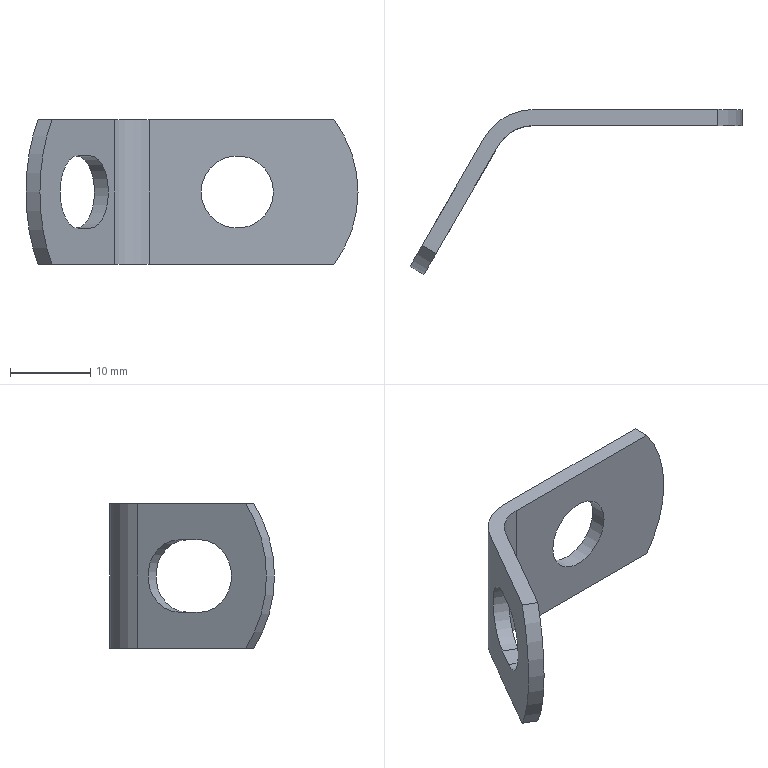Part | NX | features ACO1606-2-04 2 | 1 solid | 15 faces | box 41.25 x 20.486 x 18 mm | volume 1448 mm3 | plane 8 | cylinder 7 | commonest cylinder face diameters 9 x3 30 x2 10 x1 14 x1
STEP:
#1=CARTESIAN_POINT('',(-1007.011,-540.,-159.));
#2=VERTEX_POINT('',#1);
#3=CARTESIAN_POINT('',(-1007.011,-540.,-141.));
#4=VERTEX_POINT('',#3);
#5=CARTESIAN_POINT('',(-1007.011,-540.,-150.));
#6=DIRECTION('',(0.,0.,1.));
#7=VECTOR('',#6,1000.);
#8=LINE('',#5,#7);
#9=EDGE_CURVE('',#2,#4,#8,.T.);
#10=ORIENTED_EDGE('',*,*,#9,.T.);
#11=CARTESIAN_POINT('',(-1000.949,-536.5,-141.));
#12=VERTEX_POINT('',#11);
#13=CARTESIAN_POINT('',(-1000.949,-543.5,-141.));
#14=DIRECTION('',(0.,0.,-1.));
#15=DIRECTION('',(1.,0.,0.));
#16=AXIS2_PLACEMENT_3D('',#13,#14,#15);
#17=CIRCLE('',#16,7.);
#18=EDGE_CURVE('',#4,#12,#17,.T.);
#19=ORIENTED_EDGE('',*,*,#18,.T.);
#20=CARTESIAN_POINT('',(-1000.949,-536.5,-159.));
#21=VERTEX_POINT('',#20);
#22=CARTESIAN_POINT('',(-1000.949,-536.5,-150.));
#23=DIRECTION('',(0.,0.,1.));
#24=VECTOR('',#23,1000.);
#25=LINE('',#22,#24);
#26=EDGE_CURVE('',#21,#12,#25,.T.);
#27=ORIENTED_EDGE('',*,*,#26,.F.);
#28=CARTESIAN_POINT('',(-1000.949,-543.5,-159.));
#29=DIRECTION('',(0.,0.,-1.));
#30=DIRECTION('',(1.,0.,0.));
#31=AXIS2_PLACEMENT_3D('',#28,#29,#30);
#32=CIRCLE('',#31,7.);
#33=EDGE_CURVE('',#2,#21,#32,.T.);
#34=ORIENTED_EDGE('',*,*,#33,.F.);
#35=EDGE_LOOP('',(#10,#19,#27,#34));
#36=FACE_BOUND('',#35,.T.);
#37=CARTESIAN_POINT('',(-1000.949,-543.5,-150.));
#38=DIRECTION('',(0.,0.,1.));
#39=DIRECTION('',(1.,0.,0.));
#40=AXIS2_PLACEMENT_3D('',#37,#38,#39);
#41=CYLINDRICAL_SURFACE('',#40,7.);
#42=ADVANCED_FACE('',(#36),#41,.T.);
#43=CARTESIAN_POINT('',(-1014.74,-553.387,-159.));
#44=VERTEX_POINT('',#43);
#45=CARTESIAN_POINT('',(-1010.876,-546.694,-159.));
#46=DIRECTION('',(0.5,0.866,0.));
#47=VECTOR('',#46,1000.);
#48=LINE('',#45,#47);
#49=EDGE_CURVE('',#44,#2,#48,.T.);
#50=ORIENTED_EDGE('',*,*,#49,.F.);
#51=CARTESIAN_POINT('',(-1014.74,-553.387,-141.));
#52=VERTEX_POINT('',#51);
#53=CARTESIAN_POINT('',(-1008.74,-542.995,-150.));
#54=DIRECTION('',(0.866,-0.5,0.));
#55=DIRECTION('',(0.5,0.866,0.));
#56=AXIS2_PLACEMENT_3D('',#53,#54,#55);
#57=CIRCLE('',#56,15.);
#58=EDGE_CURVE('',#52,#44,#57,.T.);
#59=ORIENTED_EDGE('',*,*,#58,.F.);
#60=CARTESIAN_POINT('',(-1010.876,-546.694,-141.));
#61=DIRECTION('',(0.5,0.866,0.));
#62=VECTOR('',#61,1000.);
#63=LINE('',#60,#62);
#64=EDGE_CURVE('',#52,#4,#63,.T.);
#65=ORIENTED_EDGE('',*,*,#64,.T.);
#66=ORIENTED_EDGE('',*,*,#9,.F.);
#67=EDGE_LOOP('',(#50,#59,#65,#66));
#68=FACE_BOUND('',#67,.T.);
#69=CARTESIAN_POINT('',(-1011.49,-547.758,-145.5));
#70=VERTEX_POINT('',#69);
#71=CARTESIAN_POINT('',(-1009.99,-545.16,-145.5));
#72=VERTEX_POINT('',#71);
#73=CARTESIAN_POINT('',(-1010.74,-546.459,-145.5));
#74=DIRECTION('',(0.5,0.866,0.));
#75=VECTOR('',#74,1000.);
#76=LINE('',#73,#75);
#77=EDGE_CURVE('',#70,#72,#76,.T.);
#78=ORIENTED_EDGE('',*,*,#77,.F.);
#79=CARTESIAN_POINT('',(-1011.49,-547.758,-154.5));
#80=VERTEX_POINT('',#79);
#81=CARTESIAN_POINT('',(-1011.49,-547.758,-150.));
#82=DIRECTION('',(-0.866,0.5,0.));
#83=DIRECTION('',(0.5,0.866,0.));
#84=AXIS2_PLACEMENT_3D('',#81,#82,#83);
#85=CIRCLE('',#84,4.5);
#86=EDGE_CURVE('',#80,#70,#85,.T.);
#87=ORIENTED_EDGE('',*,*,#86,.F.);
#88=CARTESIAN_POINT('',(-1009.99,-545.16,-154.5));
#89=VERTEX_POINT('',#88);
#90=CARTESIAN_POINT('',(-1010.74,-546.459,-154.5));
#91=DIRECTION('',(-0.5,-0.866,0.));
#92=VECTOR('',#91,1000.);
#93=LINE('',#90,#92);
#94=EDGE_CURVE('',#89,#80,#93,.T.);
#95=ORIENTED_EDGE('',*,*,#94,.F.);
#96=CARTESIAN_POINT('',(-1009.99,-545.16,-150.));
#97=DIRECTION('',(-0.866,0.5,0.));
#98=DIRECTION('',(0.5,0.866,0.));
#99=AXIS2_PLACEMENT_3D('',#96,#97,#98);
#100=CIRCLE('',#99,4.5);
#101=EDGE_CURVE('',#72,#89,#100,.T.);
#102=ORIENTED_EDGE('',*,*,#101,.F.);
#103=EDGE_LOOP('',(#78,#87,#95,#102));
#104=FACE_BOUND('',#103,.T.);
#105=CARTESIAN_POINT('',(-1016.49,-556.419,-150.));
#106=DIRECTION('',(-0.866,0.5,0.));
#107=DIRECTION('',(0.5,0.866,0.));
#108=AXIS2_PLACEMENT_3D('',#105,#106,#107);
#109=PLANE('',#108);
#110=ADVANCED_FACE('',(#68,#104),#109,.T.);
#111=CARTESIAN_POINT('',(-977.99,-538.5,-159.));
#112=VERTEX_POINT('',#111);
#113=CARTESIAN_POINT('',(-977.99,-536.5,-159.));
#114=VERTEX_POINT('',#113);
#115=CARTESIAN_POINT('',(-977.99,-537.5,-159.));
#116=DIRECTION('',(0.,1.,0.));
#117=VECTOR('',#116,1000.);
#118=LINE('',#115,#117);
#119=EDGE_CURVE('',#112,#114,#118,.T.);
#120=ORIENTED_EDGE('',*,*,#119,.F.);
#121=CARTESIAN_POINT('',(-1000.949,-538.5,-159.));
#122=VERTEX_POINT('',#121);
#123=CARTESIAN_POINT('',(-989.47,-538.5,-159.));
#124=DIRECTION('',(-1.,0.,0.));
#125=VECTOR('',#124,1000.);
#126=LINE('',#123,#125);
#127=EDGE_CURVE('',#112,#122,#126,.T.);
#128=ORIENTED_EDGE('',*,*,#127,.T.);
#129=CARTESIAN_POINT('',(-1005.279,-541.,-159.));
#130=VERTEX_POINT('',#129);
#131=CARTESIAN_POINT('',(-1000.949,-543.5,-159.));
#132=DIRECTION('',(0.,0.,1.));
#133=DIRECTION('',(1.,0.,0.));
#134=AXIS2_PLACEMENT_3D('',#131,#132,#133);
#135=CIRCLE('',#134,5.);
#136=EDGE_CURVE('',#122,#130,#135,.T.);
#137=ORIENTED_EDGE('',*,*,#136,.T.);
#138=CARTESIAN_POINT('',(-1013.008,-554.387,-159.));
#139=VERTEX_POINT('',#138);
#140=CARTESIAN_POINT('',(-1009.144,-547.694,-159.));
#141=DIRECTION('',(-0.5,-0.866,0.));
#142=VECTOR('',#141,1000.);
#143=LINE('',#140,#142);
#144=EDGE_CURVE('',#130,#139,#143,.T.);
#145=ORIENTED_EDGE('',*,*,#144,.T.);
#146=CARTESIAN_POINT('',(-1013.874,-553.887,-159.));
#147=DIRECTION('',(-0.866,0.5,0.));
#148=VECTOR('',#147,1000.);
#149=LINE('',#146,#148);
#150=EDGE_CURVE('',#139,#44,#149,.T.);
#151=ORIENTED_EDGE('',*,*,#150,.T.);
#152=ORIENTED_EDGE('',*,*,#49,.T.);
#153=ORIENTED_EDGE('',*,*,#33,.T.);
#154=CARTESIAN_POINT('',(-989.47,-536.5,-159.));
#155=DIRECTION('',(1.,0.,0.));
#156=VECTOR('',#155,1000.);
#157=LINE('',#154,#156);
#158=EDGE_CURVE('',#21,#114,#157,.T.);
#159=ORIENTED_EDGE('',*,*,#158,.T.);
#160=EDGE_LOOP('',(#120,#128,#137,#145,#151,#152,#153,#159));
#161=FACE_BOUND('',#160,.T.);
#162=CARTESIAN_POINT('',(-1014.667,-527.579,-159.));
#163=DIRECTION('',(0.,0.,1.));
#164=DIRECTION('',(1.,0.,0.));
#165=AXIS2_PLACEMENT_3D('',#162,#163,#164);
#166=PLANE('',#165);
#167=ADVANCED_FACE('',(#161),#166,.F.);
#168=CARTESIAN_POINT('',(-977.99,-536.5,-141.));
#169=VERTEX_POINT('',#168);
#170=CARTESIAN_POINT('',(-989.99,-536.5,-150.));
#171=DIRECTION('',(0.,-1.,0.));
#172=DIRECTION('',(1.,0.,0.));
#173=AXIS2_PLACEMENT_3D('',#170,#171,#172);
#174=CIRCLE('',#173,15.);
#175=EDGE_CURVE('',#114,#169,#174,.T.);
#176=ORIENTED_EDGE('',*,*,#175,.F.);
#177=ORIENTED_EDGE('',*,*,#158,.F.);
#178=ORIENTED_EDGE('',*,*,#26,.T.);
#179=CARTESIAN_POINT('',(-989.47,-536.5,-141.));
#180=DIRECTION('',(1.,0.,0.));
#181=VECTOR('',#180,1000.);
#182=LINE('',#179,#181);
#183=EDGE_CURVE('',#12,#169,#182,.T.);
#184=ORIENTED_EDGE('',*,*,#183,.T.);
#185=EDGE_LOOP('',(#176,#177,#178,#184));
#186=FACE_BOUND('',#185,.T.);
#187=CARTESIAN_POINT('',(-985.49,-536.5,-150.));
#188=VERTEX_POINT('',#187);
#189=CARTESIAN_POINT('',(-989.99,-536.5,-150.));
#190=DIRECTION('',(0.,1.,0.));
#191=DIRECTION('',(1.,0.,0.));
#192=AXIS2_PLACEMENT_3D('',#189,#190,#191);
#193=CIRCLE('',#192,4.5);
#194=EDGE_CURVE('',#188,#188,#193,.T.);
#195=ORIENTED_EDGE('',*,*,#194,.F.);
#196=EDGE_LOOP('',(#195));
#197=FACE_BOUND('',#196,.T.);
#198=CARTESIAN_POINT('',(-1000.949,-536.5,-150.));
#199=DIRECTION('',(0.,1.,0.));
#200=DIRECTION('',(0.,0.,-1.));
#201=AXIS2_PLACEMENT_3D('',#198,#199,#200);
#202=PLANE('',#201);
#203=ADVANCED_FACE('',(#186,#197),#202,.T.);
#204=CARTESIAN_POINT('',(-977.99,-538.5,-141.));
#205=VERTEX_POINT('',#204);
#206=CARTESIAN_POINT('',(-1000.949,-538.5,-141.));
#207=VERTEX_POINT('',#206);
#208=CARTESIAN_POINT('',(-989.47,-538.5,-141.));
#209=DIRECTION('',(-1.,0.,0.));
#210=VECTOR('',#209,1000.);
#211=LINE('',#208,#210);
#212=EDGE_CURVE('',#205,#207,#211,.T.);
#213=ORIENTED_EDGE('',*,*,#212,.F.);
#214=CARTESIAN_POINT('',(-977.99,-537.5,-141.));
#215=DIRECTION('',(0.,1.,0.));
#216=VECTOR('',#215,1000.);
#217=LINE('',#214,#216);
#218=EDGE_CURVE('',#205,#169,#217,.T.);
#219=ORIENTED_EDGE('',*,*,#218,.T.);
#220=ORIENTED_EDGE('',*,*,#183,.F.);
#221=ORIENTED_EDGE('',*,*,#18,.F.);
#222=ORIENTED_EDGE('',*,*,#64,.F.);
#223=CARTESIAN_POINT('',(-1013.008,-554.387,-141.));
#224=VERTEX_POINT('',#223);
#225=CARTESIAN_POINT('',(-1013.874,-553.887,-141.));
#226=DIRECTION('',(-0.866,0.5,0.));
#227=VECTOR('',#226,1000.);
#228=LINE('',#225,#227);
#229=EDGE_CURVE('',#224,#52,#228,.T.);
#230=ORIENTED_EDGE('',*,*,#229,.F.);
#231=CARTESIAN_POINT('',(-1005.279,-541.,-141.));
#232=VERTEX_POINT('',#231);
#233=CARTESIAN_POINT('',(-1009.144,-547.694,-141.));
#234=DIRECTION('',(-0.5,-0.866,0.));
#235=VECTOR('',#234,1000.);
#236=LINE('',#233,#235);
#237=EDGE_CURVE('',#232,#224,#236,.T.);
#238=ORIENTED_EDGE('',*,*,#237,.F.);
#239=CARTESIAN_POINT('',(-1000.949,-543.5,-141.));
#240=DIRECTION('',(0.,0.,1.));
#241=DIRECTION('',(1.,0.,0.));
#242=AXIS2_PLACEMENT_3D('',#239,#240,#241);
#243=CIRCLE('',#242,5.);
#244=EDGE_CURVE('',#207,#232,#243,.T.);
#245=ORIENTED_EDGE('',*,*,#244,.F.);
#246=EDGE_LOOP('',(#213,#219,#220,#221,#222,#230,#238,#245));
#247=FACE_BOUND('',#246,.T.);
#248=CARTESIAN_POINT('',(-1014.667,-527.579,-141.));
#249=DIRECTION('',(0.,0.,1.));
#250=DIRECTION('',(1.,0.,0.));
#251=AXIS2_PLACEMENT_3D('',#248,#249,#250);
#252=PLANE('',#251);
#253=ADVANCED_FACE('',(#247),#252,.T.);
#254=ORIENTED_EDGE('',*,*,#229,.T.);
#255=ORIENTED_EDGE('',*,*,#58,.T.);
#256=ORIENTED_EDGE('',*,*,#150,.F.);
#257=CARTESIAN_POINT('',(-1007.008,-543.995,-150.));
#258=DIRECTION('',(0.866,-0.5,0.));
#259=DIRECTION('',(0.5,0.866,0.));
#260=AXIS2_PLACEMENT_3D('',#257,#258,#259);
#261=CIRCLE('',#260,15.);
#262=EDGE_CURVE('',#224,#139,#261,.T.);
#263=ORIENTED_EDGE('',*,*,#262,.F.);
#264=EDGE_LOOP('',(#254,#255,#256,#263));
#265=FACE_BOUND('',#264,.T.);
#266=CARTESIAN_POINT('',(-1007.874,-543.495,-150.));
#267=DIRECTION('',(0.866,-0.5,0.));
#268=DIRECTION('',(-0.5,-0.866,0.));
#269=AXIS2_PLACEMENT_3D('',#266,#267,#268);
#270=CYLINDRICAL_SURFACE('',#269,15.);
#271=ADVANCED_FACE('',(#265),#270,.T.);
#272=CARTESIAN_POINT('',(-1009.758,-548.758,-145.5));
#273=VERTEX_POINT('',#272);
#274=CARTESIAN_POINT('',(-1010.624,-548.258,-145.5));
#275=DIRECTION('',(-0.866,0.5,0.));
#276=VECTOR('',#275,1000.);
#277=LINE('',#274,#276);
#278=EDGE_CURVE('',#273,#70,#277,.T.);
#279=ORIENTED_EDGE('',*,*,#278,.T.);
#280=ORIENTED_EDGE('',*,*,#77,.T.);
#281=CARTESIAN_POINT('',(-1008.258,-546.16,-145.5));
#282=VERTEX_POINT('',#281);
#283=CARTESIAN_POINT('',(-1009.124,-545.66,-145.5));
#284=DIRECTION('',(-0.866,0.5,0.));
#285=VECTOR('',#284,1000.);
#286=LINE('',#283,#285);
#287=EDGE_CURVE('',#282,#72,#286,.T.);
#288=ORIENTED_EDGE('',*,*,#287,.F.);
#289=CARTESIAN_POINT('',(-1009.008,-547.459,-145.5));
#290=DIRECTION('',(0.5,0.866,0.));
#291=VECTOR('',#290,1000.);
#292=LINE('',#289,#291);
#293=EDGE_CURVE('',#273,#282,#292,.T.);
#294=ORIENTED_EDGE('',*,*,#293,.F.);
#295=EDGE_LOOP('',(#279,#280,#288,#294));
#296=FACE_BOUND('',#295,.T.);
#297=CARTESIAN_POINT('',(-1008.258,-546.16,-145.5));
#298=DIRECTION('',(0.,0.,1.));
#299=DIRECTION('',(1.,0.,0.));
#300=AXIS2_PLACEMENT_3D('',#297,#298,#299);
#301=PLANE('',#300);
#302=ADVANCED_FACE('',(#296),#301,.F.);
#303=ORIENTED_EDGE('',*,*,#287,.T.);
#304=ORIENTED_EDGE('',*,*,#101,.T.);
#305=CARTESIAN_POINT('',(-1008.258,-546.16,-154.5));
#306=VERTEX_POINT('',#305);
#307=CARTESIAN_POINT('',(-1009.124,-545.66,-154.5));
#308=DIRECTION('',(-0.866,0.5,0.));
#309=VECTOR('',#308,1000.);
#310=LINE('',#307,#309);
#311=EDGE_CURVE('',#306,#89,#310,.T.);
#312=ORIENTED_EDGE('',*,*,#311,.F.);
#313=CARTESIAN_POINT('',(-1008.258,-546.16,-150.));
#314=DIRECTION('',(-0.866,0.5,0.));
#315=DIRECTION('',(0.5,0.866,0.));
#316=AXIS2_PLACEMENT_3D('',#313,#314,#315);
#317=CIRCLE('',#316,4.5);
#318=EDGE_CURVE('',#282,#306,#317,.T.);
#319=ORIENTED_EDGE('',*,*,#318,.F.);
#320=EDGE_LOOP('',(#303,#304,#312,#319));
#321=FACE_BOUND('',#320,.T.);
#322=CARTESIAN_POINT('',(-1009.124,-545.66,-150.));
#323=DIRECTION('',(0.866,-0.5,0.));
#324=DIRECTION('',(-0.5,-0.866,0.));
#325=AXIS2_PLACEMENT_3D('',#322,#323,#324);
#326=CYLINDRICAL_SURFACE('',#325,4.5);
#327=ADVANCED_FACE('',(#321),#326,.F.);
#328=ORIENTED_EDGE('',*,*,#311,.T.);
#329=ORIENTED_EDGE('',*,*,#94,.T.);
#330=CARTESIAN_POINT('',(-1009.758,-548.758,-154.5));
#331=VERTEX_POINT('',#330);
#332=CARTESIAN_POINT('',(-1010.624,-548.258,-154.5));
#333=DIRECTION('',(-0.866,0.5,0.));
#334=VECTOR('',#333,1000.);
#335=LINE('',#332,#334);
#336=EDGE_CURVE('',#331,#80,#335,.T.);
#337=ORIENTED_EDGE('',*,*,#336,.F.);
#338=CARTESIAN_POINT('',(-1009.008,-547.459,-154.5));
#339=DIRECTION('',(-0.5,-0.866,0.));
#340=VECTOR('',#339,1000.);
#341=LINE('',#338,#340);
#342=EDGE_CURVE('',#306,#331,#341,.T.);
#343=ORIENTED_EDGE('',*,*,#342,.F.);
#344=EDGE_LOOP('',(#328,#329,#337,#343));
#345=FACE_BOUND('',#344,.T.);
#346=CARTESIAN_POINT('',(-1009.758,-548.758,-154.5));
#347=DIRECTION('',(0.,0.,-1.));
#348=DIRECTION('',(-1.,0.,0.));
#349=AXIS2_PLACEMENT_3D('',#346,#347,#348);
#350=PLANE('',#349);
#351=ADVANCED_FACE('',(#345),#350,.F.);
#352=ORIENTED_EDGE('',*,*,#336,.T.);
#353=ORIENTED_EDGE('',*,*,#86,.T.);
#354=ORIENTED_EDGE('',*,*,#278,.F.);
#355=CARTESIAN_POINT('',(-1009.758,-548.758,-150.));
#356=DIRECTION('',(-0.866,0.5,0.));
#357=DIRECTION('',(0.5,0.866,0.));
#358=AXIS2_PLACEMENT_3D('',#355,#356,#357);
#359=CIRCLE('',#358,4.5);
#360=EDGE_CURVE('',#331,#273,#359,.T.);
#361=ORIENTED_EDGE('',*,*,#360,.F.);
#362=EDGE_LOOP('',(#352,#353,#354,#361));
#363=FACE_BOUND('',#362,.T.);
#364=CARTESIAN_POINT('',(-1010.624,-548.258,-150.));
#365=DIRECTION('',(0.866,-0.5,0.));
#366=DIRECTION('',(-0.5,-0.866,0.));
#367=AXIS2_PLACEMENT_3D('',#364,#365,#366);
#368=CYLINDRICAL_SURFACE('',#367,4.5);
#369=ADVANCED_FACE('',(#363),#368,.F.);
#370=ORIENTED_EDGE('',*,*,#127,.F.);
#371=CARTESIAN_POINT('',(-989.99,-538.5,-150.));
#372=DIRECTION('',(0.,-1.,0.));
#373=DIRECTION('',(1.,0.,0.));
#374=AXIS2_PLACEMENT_3D('',#371,#372,#373);
#375=CIRCLE('',#374,15.);
#376=EDGE_CURVE('',#112,#205,#375,.T.);
#377=ORIENTED_EDGE('',*,*,#376,.T.);
#378=ORIENTED_EDGE('',*,*,#212,.T.);
#379=CARTESIAN_POINT('',(-1000.949,-538.5,-150.));
#380=DIRECTION('',(0.,0.,1.));
#381=VECTOR('',#380,1000.);
#382=LINE('',#379,#381);
#383=EDGE_CURVE('',#122,#207,#382,.T.);
#384=ORIENTED_EDGE('',*,*,#383,.F.);
#385=EDGE_LOOP('',(#370,#377,#378,#384));
#386=FACE_BOUND('',#385,.T.);
#387=CARTESIAN_POINT('',(-985.49,-538.5,-150.));
#388=VERTEX_POINT('',#387);
#389=CARTESIAN_POINT('',(-989.99,-538.5,-150.));
#390=DIRECTION('',(0.,1.,0.));
#391=DIRECTION('',(1.,0.,0.));
#392=AXIS2_PLACEMENT_3D('',#389,#390,#391);
#393=CIRCLE('',#392,4.5);
#394=EDGE_CURVE('',#388,#388,#393,.T.);
#395=ORIENTED_EDGE('',*,*,#394,.T.);
#396=EDGE_LOOP('',(#395));
#397=FACE_BOUND('',#396,.T.);
#398=CARTESIAN_POINT('',(-974.99,-538.5,-150.));
#399=DIRECTION('',(0.,-1.,0.));
#400=DIRECTION('',(0.,0.,1.));
#401=AXIS2_PLACEMENT_3D('',#398,#399,#400);
#402=PLANE('',#401);
#403=ADVANCED_FACE('',(#386,#397),#402,.T.);
#404=ORIENTED_EDGE('',*,*,#383,.T.);
#405=ORIENTED_EDGE('',*,*,#244,.T.);
#406=CARTESIAN_POINT('',(-1005.279,-541.,-150.));
#407=DIRECTION('',(0.,0.,1.));
#408=VECTOR('',#407,1000.);
#409=LINE('',#406,#408);
#410=EDGE_CURVE('',#130,#232,#409,.T.);
#411=ORIENTED_EDGE('',*,*,#410,.F.);
#412=ORIENTED_EDGE('',*,*,#136,.F.);
#413=EDGE_LOOP('',(#404,#405,#411,#412));
#414=FACE_BOUND('',#413,.T.);
#415=CARTESIAN_POINT('',(-1000.949,-543.5,-150.));
#416=DIRECTION('',(0.,0.,1.));
#417=DIRECTION('',(1.,0.,0.));
#418=AXIS2_PLACEMENT_3D('',#415,#416,#417);
#419=CYLINDRICAL_SURFACE('',#418,5.);
#420=ADVANCED_FACE('',(#414),#419,.F.);
#421=ORIENTED_EDGE('',*,*,#262,.T.);
#422=ORIENTED_EDGE('',*,*,#144,.F.);
#423=ORIENTED_EDGE('',*,*,#410,.T.);
#424=ORIENTED_EDGE('',*,*,#237,.T.);
#425=EDGE_LOOP('',(#421,#422,#423,#424));
#426=FACE_BOUND('',#425,.T.);
#427=ORIENTED_EDGE('',*,*,#360,.T.);
#428=ORIENTED_EDGE('',*,*,#293,.T.);
#429=ORIENTED_EDGE('',*,*,#318,.T.);
#430=ORIENTED_EDGE('',*,*,#342,.T.);
#431=EDGE_LOOP('',(#427,#428,#429,#430));
#432=FACE_BOUND('',#431,.T.);
#433=CARTESIAN_POINT('',(-1014.758,-557.419,-150.));
#434=DIRECTION('',(-0.866,0.5,0.));
#435=DIRECTION('',(0.5,0.866,0.));
#436=AXIS2_PLACEMENT_3D('',#433,#434,#435);
#437=PLANE('',#436);
#438=ADVANCED_FACE('',(#426,#432),#437,.F.);
#439=ORIENTED_EDGE('',*,*,#194,.T.);
#440=EDGE_LOOP('',(#439));
#441=FACE_BOUND('',#440,.T.);
#442=ORIENTED_EDGE('',*,*,#394,.F.);
#443=EDGE_LOOP('',(#442));
#444=FACE_BOUND('',#443,.T.);
#445=CARTESIAN_POINT('',(-989.99,-537.5,-150.));
#446=DIRECTION('',(0.,-1.,0.));
#447=DIRECTION('',(0.,0.,1.));
#448=AXIS2_PLACEMENT_3D('',#445,#446,#447);
#449=CYLINDRICAL_SURFACE('',#448,4.5);
#450=ADVANCED_FACE('',(#441,#444),#449,.F.);
#451=ORIENTED_EDGE('',*,*,#175,.T.);
#452=ORIENTED_EDGE('',*,*,#218,.F.);
#453=ORIENTED_EDGE('',*,*,#376,.F.);
#454=ORIENTED_EDGE('',*,*,#119,.T.);
#455=EDGE_LOOP('',(#451,#452,#453,#454));
#456=FACE_BOUND('',#455,.T.);
#457=CARTESIAN_POINT('',(-989.99,-537.5,-150.));
#458=DIRECTION('',(0.,-1.,0.));
#459=DIRECTION('',(0.,0.,1.));
#460=AXIS2_PLACEMENT_3D('',#457,#458,#459);
#461=CYLINDRICAL_SURFACE('',#460,15.);
#462=ADVANCED_FACE('',(#456),#461,.T.);
#463=CLOSED_SHELL('',(#42,#110,#167,#203,#253,#271,#302,#327,#351,#369,#403,#420,#438,#450,#462));
#464=MANIFOLD_SOLID_BREP('',#463);
#465=(LENGTH_UNIT()NAMED_UNIT(*)SI_UNIT(.MILLI.,.METRE.));
#466=UNCERTAINTY_MEASURE_WITH_UNIT(LENGTH_MEASURE(0.00001),#465,'','');
#467=(NAMED_UNIT(*)PLANE_ANGLE_UNIT()SI_UNIT($,.RADIAN.));
#468=(NAMED_UNIT(*)SI_UNIT($,.STERADIAN.)SOLID_ANGLE_UNIT());
#469=(GEOMETRIC_REPRESENTATION_CONTEXT(3)GLOBAL_UNCERTAINTY_ASSIGNED_CONTEXT((#466))GLOBAL_UNIT_ASSIGNED_CONTEXT((#465,#467,#468))REPRESENTATION_CONTEXT('',''));
#470=ADVANCED_BREP_SHAPE_REPRESENTATION('',(#464),#469);